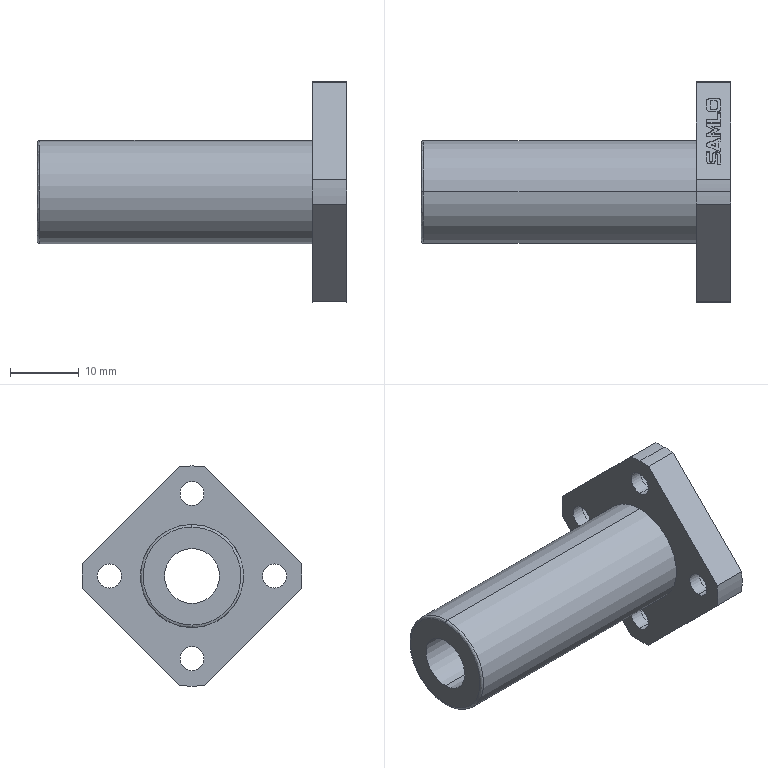Part | SolidWorks | features BaseBody 1 | 1 solid | 104 faces | box 45 x 32 x 32 mm | volume 7447 mm3 | plane 63 | cylinder 39 | spline 2 | commonest cylinder face diameters 3.5 x8 6 x8 32 x5 0.459 x4 0.974 x4 0.329 x3